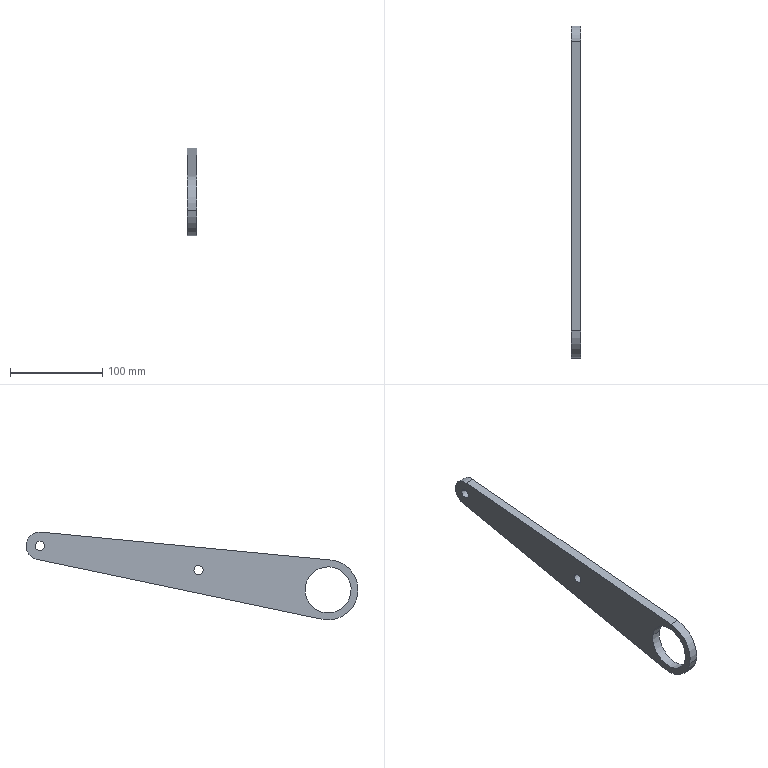Part | NX | features _-17372000 2 | 1 solid | 13 faces | box 10 x 359.893 x 95.107 mm | volume 149250 mm3 | cylinder 9 | plane 4 | commonest cylinder face diameters 10 x4 50 x2 65 x2 30 x1
STEP:
#1=CARTESIAN_POINT('',(-12.5,-285.515,-699.296));
#2=VERTEX_POINT('',#1);
#3=CARTESIAN_POINT('',(-12.5,-236.085,-691.763));
#4=VERTEX_POINT('',#3);
#5=CARTESIAN_POINT('',(-12.5,-260.8,-695.529));
#6=DIRECTION('',(1.,0.,0.));
#7=DIRECTION('',(0.,-0.9886,-0.1507));
#8=AXIS2_PLACEMENT_3D('',#5,#6,#7);
#9=CIRCLE('',#8,25.);
#10=EDGE_CURVE('',#2,#4,#9,.T.);
#11=ORIENTED_EDGE('',*,*,#10,.F.);
#12=CARTESIAN_POINT('',(-2.5,-285.515,-699.296));
#13=VERTEX_POINT('',#12);
#14=CARTESIAN_POINT('',(-2.5,-285.515,-699.296));
#15=DIRECTION('',(-1.,0.,0.));
#16=VECTOR('',#15,1000.);
#17=LINE('',#14,#16);
#18=EDGE_CURVE('',#2,#13,#17,.F.);
#19=ORIENTED_EDGE('',*,*,#18,.T.);
#20=CARTESIAN_POINT('',(-2.5,-236.085,-691.763));
#21=VERTEX_POINT('',#20);
#22=CARTESIAN_POINT('',(-2.5,-260.8,-695.529));
#23=DIRECTION('',(-1.,0.,0.));
#24=DIRECTION('',(0.,0.9886,0.1507));
#25=AXIS2_PLACEMENT_3D('',#22,#23,#24);
#26=CIRCLE('',#25,25.);
#27=EDGE_CURVE('',#21,#13,#26,.T.);
#28=ORIENTED_EDGE('',*,*,#27,.F.);
#29=CARTESIAN_POINT('',(-2.5,-236.085,-691.763));
#30=DIRECTION('',(-1.,0.,0.));
#31=VECTOR('',#30,1000.);
#32=LINE('',#29,#31);
#33=EDGE_CURVE('',#21,#4,#32,.T.);
#34=ORIENTED_EDGE('',*,*,#33,.T.);
#35=EDGE_LOOP('',(#11,#19,#28,#34));
#36=FACE_BOUND('',#35,.T.);
#37=CARTESIAN_POINT('',(-12.5,-260.8,-695.529));
#38=DIRECTION('',(1.,0.,0.));
#39=DIRECTION('',(0.,-0.9886,-0.1507));
#40=AXIS2_PLACEMENT_3D('',#37,#38,#39);
#41=CYLINDRICAL_SURFACE('',#40,25.);
#42=ADVANCED_FACE('',(#36),#41,.F.);
#43=ORIENTED_EDGE('',*,*,#33,.F.);
#44=CARTESIAN_POINT('',(-2.5,-260.8,-695.529));
#45=DIRECTION('',(-1.,0.,0.));
#46=DIRECTION('',(0.,-0.9886,-0.1507));
#47=AXIS2_PLACEMENT_3D('',#44,#45,#46);
#48=CIRCLE('',#47,25.);
#49=EDGE_CURVE('',#13,#21,#48,.T.);
#50=ORIENTED_EDGE('',*,*,#49,.F.);
#51=ORIENTED_EDGE('',*,*,#18,.F.);
#52=CARTESIAN_POINT('',(-12.5,-260.8,-695.529));
#53=DIRECTION('',(1.,0.,0.));
#54=DIRECTION('',(0.,0.9886,0.1507));
#55=AXIS2_PLACEMENT_3D('',#52,#53,#54);
#56=CIRCLE('',#55,25.);
#57=EDGE_CURVE('',#4,#2,#56,.T.);
#58=ORIENTED_EDGE('',*,*,#57,.F.);
#59=EDGE_LOOP('',(#43,#50,#51,#58));
#60=FACE_BOUND('',#59,.T.);
#61=CARTESIAN_POINT('',(-12.5,-260.8,-695.529));
#62=DIRECTION('',(1.,0.,0.));
#63=DIRECTION('',(0.,-0.9886,-0.1507));
#64=AXIS2_PLACEMENT_3D('',#61,#62,#63);
#65=CYLINDRICAL_SURFACE('',#64,25.);
#66=ADVANCED_FACE('',(#60),#65,.F.);
#67=CARTESIAN_POINT('',(-12.5,-125.364,-674.89));
#68=VERTEX_POINT('',#67);
#69=CARTESIAN_POINT('',(-12.5,-115.478,-673.383));
#70=VERTEX_POINT('',#69);
#71=CARTESIAN_POINT('',(-12.5,-120.421,-674.136));
#72=DIRECTION('',(1.,0.,0.));
#73=DIRECTION('',(0.,-0.9886,-0.1507));
#74=AXIS2_PLACEMENT_3D('',#71,#72,#73);
#75=CIRCLE('',#74,5.);
#76=EDGE_CURVE('',#68,#70,#75,.T.);
#77=ORIENTED_EDGE('',*,*,#76,.F.);
#78=CARTESIAN_POINT('',(-2.5,-125.364,-674.89));
#79=VERTEX_POINT('',#78);
#80=CARTESIAN_POINT('',(-2.5,-125.364,-674.89));
#81=DIRECTION('',(-1.,0.,0.));
#82=VECTOR('',#81,1000.);
#83=LINE('',#80,#82);
#84=EDGE_CURVE('',#68,#79,#83,.F.);
#85=ORIENTED_EDGE('',*,*,#84,.T.);
#86=CARTESIAN_POINT('',(-2.5,-115.478,-673.383));
#87=VERTEX_POINT('',#86);
#88=CARTESIAN_POINT('',(-2.5,-120.421,-674.136));
#89=DIRECTION('',(-1.,0.,0.));
#90=DIRECTION('',(0.,0.9886,0.1507));
#91=AXIS2_PLACEMENT_3D('',#88,#89,#90);
#92=CIRCLE('',#91,5.);
#93=EDGE_CURVE('',#87,#79,#92,.T.);
#94=ORIENTED_EDGE('',*,*,#93,.F.);
#95=CARTESIAN_POINT('',(-2.5,-115.478,-673.383));
#96=DIRECTION('',(-1.,0.,0.));
#97=VECTOR('',#96,1000.);
#98=LINE('',#95,#97);
#99=EDGE_CURVE('',#87,#70,#98,.T.);
#100=ORIENTED_EDGE('',*,*,#99,.T.);
#101=EDGE_LOOP('',(#77,#85,#94,#100));
#102=FACE_BOUND('',#101,.T.);
#103=CARTESIAN_POINT('',(-12.5,-120.421,-674.136));
#104=DIRECTION('',(1.,0.,0.));
#105=DIRECTION('',(0.,-0.9886,-0.1507));
#106=AXIS2_PLACEMENT_3D('',#103,#104,#105);
#107=CYLINDRICAL_SURFACE('',#106,5.);
#108=ADVANCED_FACE('',(#102),#107,.F.);
#109=ORIENTED_EDGE('',*,*,#99,.F.);
#110=CARTESIAN_POINT('',(-2.5,-120.421,-674.136));
#111=DIRECTION('',(-1.,0.,0.));
#112=DIRECTION('',(0.,-0.9886,-0.1507));
#113=AXIS2_PLACEMENT_3D('',#110,#111,#112);
#114=CIRCLE('',#113,5.);
#115=EDGE_CURVE('',#79,#87,#114,.T.);
#116=ORIENTED_EDGE('',*,*,#115,.F.);
#117=ORIENTED_EDGE('',*,*,#84,.F.);
#118=CARTESIAN_POINT('',(-12.5,-120.421,-674.136));
#119=DIRECTION('',(1.,0.,0.));
#120=DIRECTION('',(0.,0.9886,0.1507));
#121=AXIS2_PLACEMENT_3D('',#118,#119,#120);
#122=CIRCLE('',#121,5.);
#123=EDGE_CURVE('',#70,#68,#122,.T.);
#124=ORIENTED_EDGE('',*,*,#123,.F.);
#125=EDGE_LOOP('',(#109,#116,#117,#124));
#126=FACE_BOUND('',#125,.T.);
#127=CARTESIAN_POINT('',(-12.5,-120.421,-674.136));
#128=DIRECTION('',(1.,0.,0.));
#129=DIRECTION('',(0.,-0.9886,-0.1507));
#130=AXIS2_PLACEMENT_3D('',#127,#128,#129);
#131=CYLINDRICAL_SURFACE('',#130,5.);
#132=ADVANCED_FACE('',(#126),#131,.F.);
#133=CARTESIAN_POINT('',(-12.5,46.65,-648.676));
#134=VERTEX_POINT('',#133);
#135=CARTESIAN_POINT('',(-12.5,56.536,-647.169));
#136=VERTEX_POINT('',#135);
#137=CARTESIAN_POINT('',(-12.5,51.593,-647.922));
#138=DIRECTION('',(1.,0.,0.));
#139=DIRECTION('',(0.,-0.9886,-0.1507));
#140=AXIS2_PLACEMENT_3D('',#137,#138,#139);
#141=CIRCLE('',#140,5.);
#142=EDGE_CURVE('',#134,#136,#141,.T.);
#143=ORIENTED_EDGE('',*,*,#142,.F.);
#144=CARTESIAN_POINT('',(-2.5,46.65,-648.676));
#145=VERTEX_POINT('',#144);
#146=CARTESIAN_POINT('',(-2.5,46.65,-648.676));
#147=DIRECTION('',(-1.,0.,0.));
#148=VECTOR('',#147,1000.);
#149=LINE('',#146,#148);
#150=EDGE_CURVE('',#145,#134,#149,.T.);
#151=ORIENTED_EDGE('',*,*,#150,.F.);
#152=CARTESIAN_POINT('',(-2.5,56.536,-647.169));
#153=VERTEX_POINT('',#152);
#154=CARTESIAN_POINT('',(-2.5,51.593,-647.922));
#155=DIRECTION('',(-1.,0.,0.));
#156=DIRECTION('',(0.,0.9886,0.1507));
#157=AXIS2_PLACEMENT_3D('',#154,#155,#156);
#158=CIRCLE('',#157,5.);
#159=EDGE_CURVE('',#153,#145,#158,.T.);
#160=ORIENTED_EDGE('',*,*,#159,.F.);
#161=CARTESIAN_POINT('',(-2.5,56.536,-647.169));
#162=DIRECTION('',(-1.,0.,0.));
#163=VECTOR('',#162,1000.);
#164=LINE('',#161,#163);
#165=EDGE_CURVE('',#136,#153,#164,.F.);
#166=ORIENTED_EDGE('',*,*,#165,.F.);
#167=EDGE_LOOP('',(#143,#151,#160,#166));
#168=FACE_BOUND('',#167,.T.);
#169=CARTESIAN_POINT('',(-12.5,51.593,-647.922));
#170=DIRECTION('',(1.,0.,0.));
#171=DIRECTION('',(0.,-0.9886,-0.1507));
#172=AXIS2_PLACEMENT_3D('',#169,#170,#171);
#173=CYLINDRICAL_SURFACE('',#172,5.);
#174=ADVANCED_FACE('',(#168),#173,.F.);
#175=ORIENTED_EDGE('',*,*,#165,.T.);
#176=CARTESIAN_POINT('',(-2.5,51.593,-647.922));
#177=DIRECTION('',(-1.,0.,0.));
#178=DIRECTION('',(0.,-0.9886,-0.1507));
#179=AXIS2_PLACEMENT_3D('',#176,#177,#178);
#180=CIRCLE('',#179,5.);
#181=EDGE_CURVE('',#145,#153,#180,.T.);
#182=ORIENTED_EDGE('',*,*,#181,.F.);
#183=ORIENTED_EDGE('',*,*,#150,.T.);
#184=CARTESIAN_POINT('',(-12.5,51.593,-647.922));
#185=DIRECTION('',(1.,0.,0.));
#186=DIRECTION('',(0.,0.9886,0.1507));
#187=AXIS2_PLACEMENT_3D('',#184,#185,#186);
#188=CIRCLE('',#187,5.);
#189=EDGE_CURVE('',#136,#134,#188,.T.);
#190=ORIENTED_EDGE('',*,*,#189,.F.);
#191=EDGE_LOOP('',(#175,#182,#183,#190));
#192=FACE_BOUND('',#191,.T.);
#193=CARTESIAN_POINT('',(-12.5,51.593,-647.922));
#194=DIRECTION('',(1.,0.,0.));
#195=DIRECTION('',(0.,-0.9886,-0.1507));
#196=AXIS2_PLACEMENT_3D('',#193,#194,#195);
#197=CYLINDRICAL_SURFACE('',#196,5.);
#198=ADVANCED_FACE('',(#192),#197,.F.);
#199=CARTESIAN_POINT('',(-12.5,-254.132,-727.338));
#200=VERTEX_POINT('',#199);
#201=CARTESIAN_POINT('',(-2.5,-254.132,-727.338));
#202=VERTEX_POINT('',#201);
#203=CARTESIAN_POINT('',(-12.5,-254.132,-727.338));
#204=DIRECTION('',(1.,0.,0.));
#205=VECTOR('',#204,1000.);
#206=LINE('',#203,#205);
#207=EDGE_CURVE('',#200,#202,#206,.T.);
#208=ORIENTED_EDGE('',*,*,#207,.F.);
#209=CARTESIAN_POINT('',(-12.5,54.671,-662.603));
#210=VERTEX_POINT('',#209);
#211=CARTESIAN_POINT('',(-12.5,54.671,-662.603));
#212=DIRECTION('',(0.,-0.9787,-0.2052));
#213=VECTOR('',#212,1000.);
#214=LINE('',#211,#213);
#215=EDGE_CURVE('',#210,#200,#214,.T.);
#216=ORIENTED_EDGE('',*,*,#215,.F.);
#217=CARTESIAN_POINT('',(-2.5,54.671,-662.603));
#218=VERTEX_POINT('',#217);
#219=CARTESIAN_POINT('',(-2.5,54.671,-662.603));
#220=DIRECTION('',(-1.,0.,0.));
#221=VECTOR('',#220,1000.);
#222=LINE('',#219,#221);
#223=EDGE_CURVE('',#218,#210,#222,.T.);
#224=ORIENTED_EDGE('',*,*,#223,.F.);
#225=CARTESIAN_POINT('',(-2.5,-254.132,-727.338));
#226=DIRECTION('',(0.,0.9787,0.2052));
#227=VECTOR('',#226,1000.);
#228=LINE('',#225,#227);
#229=EDGE_CURVE('',#202,#218,#228,.T.);
#230=ORIENTED_EDGE('',*,*,#229,.F.);
#231=EDGE_LOOP('',(#208,#216,#224,#230));
#232=FACE_BOUND('',#231,.T.);
#233=CARTESIAN_POINT('',(-12.5,54.671,-662.603));
#234=DIRECTION('',(0.,-0.2052,0.9787));
#235=DIRECTION('',(0.,0.9787,0.2052));
#236=AXIS2_PLACEMENT_3D('',#233,#234,#235);
#237=PLANE('',#236);
#238=ADVANCED_FACE('',(#232),#237,.F.);
#239=ORIENTED_EDGE('',*,*,#223,.T.);
#240=CARTESIAN_POINT('',(-12.5,50.158,-632.991));
#241=VERTEX_POINT('',#240);
#242=CARTESIAN_POINT('',(-12.5,51.593,-647.922));
#243=DIRECTION('',(-1.,0.,0.));
#244=DIRECTION('',(0.,-0.09568,0.9954));
#245=AXIS2_PLACEMENT_3D('',#242,#243,#244);
#246=CIRCLE('',#245,15.);
#247=EDGE_CURVE('',#241,#210,#246,.T.);
#248=ORIENTED_EDGE('',*,*,#247,.F.);
#249=CARTESIAN_POINT('',(-2.5,50.158,-632.991));
#250=VERTEX_POINT('',#249);
#251=CARTESIAN_POINT('',(-12.5,50.158,-632.991));
#252=DIRECTION('',(1.,0.,0.));
#253=VECTOR('',#252,1000.);
#254=LINE('',#251,#253);
#255=EDGE_CURVE('',#241,#250,#254,.T.);
#256=ORIENTED_EDGE('',*,*,#255,.T.);
#257=CARTESIAN_POINT('',(-2.5,51.593,-647.922));
#258=DIRECTION('',(1.,0.,0.));
#259=DIRECTION('',(0.,0.2052,-0.9787));
#260=AXIS2_PLACEMENT_3D('',#257,#258,#259);
#261=CIRCLE('',#260,15.);
#262=EDGE_CURVE('',#218,#250,#261,.T.);
#263=ORIENTED_EDGE('',*,*,#262,.F.);
#264=EDGE_LOOP('',(#239,#248,#256,#263));
#265=FACE_BOUND('',#264,.T.);
#266=CARTESIAN_POINT('',(-12.5,51.593,-647.922));
#267=DIRECTION('',(1.,0.,0.));
#268=DIRECTION('',(0.,-0.9886,-0.1507));
#269=AXIS2_PLACEMENT_3D('',#266,#267,#268);
#270=CYLINDRICAL_SURFACE('',#269,15.);
#271=ADVANCED_FACE('',(#265),#270,.T.);
#272=ORIENTED_EDGE('',*,*,#27,.T.);
#273=ORIENTED_EDGE('',*,*,#49,.T.);
#274=EDGE_LOOP('',(#272,#273));
#275=FACE_BOUND('',#274,.T.);
#276=ORIENTED_EDGE('',*,*,#93,.T.);
#277=ORIENTED_EDGE('',*,*,#115,.T.);
#278=EDGE_LOOP('',(#276,#277));
#279=FACE_BOUND('',#278,.T.);
#280=ORIENTED_EDGE('',*,*,#159,.T.);
#281=ORIENTED_EDGE('',*,*,#181,.T.);
#282=EDGE_LOOP('',(#280,#281));
#283=FACE_BOUND('',#282,.T.);
#284=ORIENTED_EDGE('',*,*,#229,.T.);
#285=ORIENTED_EDGE('',*,*,#262,.T.);
#286=CARTESIAN_POINT('',(-2.5,-263.909,-663.179));
#287=VERTEX_POINT('',#286);
#288=CARTESIAN_POINT('',(-2.5,50.158,-632.991));
#289=DIRECTION('',(0.,-0.9954,-0.09568));
#290=VECTOR('',#289,1000.);
#291=LINE('',#288,#290);
#292=EDGE_CURVE('',#250,#287,#291,.T.);
#293=ORIENTED_EDGE('',*,*,#292,.T.);
#294=CARTESIAN_POINT('',(-2.5,-292.929,-700.426));
#295=VERTEX_POINT('',#294);
#296=CARTESIAN_POINT('',(-2.5,-260.8,-695.529));
#297=DIRECTION('',(1.,0.,0.));
#298=DIRECTION('',(0.,-0.09568,0.9954));
#299=AXIS2_PLACEMENT_3D('',#296,#297,#298);
#300=CIRCLE('',#299,32.5);
#301=EDGE_CURVE('',#287,#295,#300,.T.);
#302=ORIENTED_EDGE('',*,*,#301,.T.);
#303=CARTESIAN_POINT('',(-2.5,-260.8,-695.529));
#304=DIRECTION('',(1.,0.,0.));
#305=DIRECTION('',(0.,-0.9886,-0.1507));
#306=AXIS2_PLACEMENT_3D('',#303,#304,#305);
#307=CIRCLE('',#306,32.5);
#308=EDGE_CURVE('',#295,#202,#307,.T.);
#309=ORIENTED_EDGE('',*,*,#308,.T.);
#310=EDGE_LOOP('',(#284,#285,#293,#302,#309));
#311=FACE_BOUND('',#310,.T.);
#312=CARTESIAN_POINT('',(-2.5,-260.8,-695.529));
#313=DIRECTION('',(-1.,0.,0.));
#314=DIRECTION('',(0.,0.9886,0.1507));
#315=AXIS2_PLACEMENT_3D('',#312,#313,#314);
#316=PLANE('',#315);
#317=ADVANCED_FACE('',(#275,#279,#283,#311),#316,.F.);
#318=ORIENTED_EDGE('',*,*,#255,.F.);
#319=CARTESIAN_POINT('',(-12.5,-263.909,-663.179));
#320=VERTEX_POINT('',#319);
#321=CARTESIAN_POINT('',(-12.5,-263.909,-663.179));
#322=DIRECTION('',(0.,0.9954,0.09568));
#323=VECTOR('',#322,1000.);
#324=LINE('',#321,#323);
#325=EDGE_CURVE('',#320,#241,#324,.T.);
#326=ORIENTED_EDGE('',*,*,#325,.F.);
#327=CARTESIAN_POINT('',(-2.5,-263.909,-663.179));
#328=DIRECTION('',(-1.,0.,0.));
#329=VECTOR('',#328,1000.);
#330=LINE('',#327,#329);
#331=EDGE_CURVE('',#287,#320,#330,.T.);
#332=ORIENTED_EDGE('',*,*,#331,.F.);
#333=ORIENTED_EDGE('',*,*,#292,.F.);
#334=EDGE_LOOP('',(#318,#326,#332,#333));
#335=FACE_BOUND('',#334,.T.);
#336=CARTESIAN_POINT('',(-12.5,-263.909,-663.179));
#337=DIRECTION('',(0.,0.09568,-0.9954));
#338=DIRECTION('',(0.,-0.9954,-0.09568));
#339=AXIS2_PLACEMENT_3D('',#336,#337,#338);
#340=PLANE('',#339);
#341=ADVANCED_FACE('',(#335),#340,.F.);
#342=CARTESIAN_POINT('',(-12.5,-292.929,-700.426));
#343=VERTEX_POINT('',#342);
#344=CARTESIAN_POINT('',(-2.5,-292.929,-700.426));
#345=DIRECTION('',(-1.,0.,0.));
#346=VECTOR('',#345,1000.);
#347=LINE('',#344,#346);
#348=EDGE_CURVE('',#295,#343,#347,.T.);
#349=ORIENTED_EDGE('',*,*,#348,.F.);
#350=ORIENTED_EDGE('',*,*,#301,.F.);
#351=ORIENTED_EDGE('',*,*,#331,.T.);
#352=CARTESIAN_POINT('',(-12.5,-260.8,-695.529));
#353=DIRECTION('',(-1.,0.,0.));
#354=DIRECTION('',(0.,-0.9886,-0.1507));
#355=AXIS2_PLACEMENT_3D('',#352,#353,#354);
#356=CIRCLE('',#355,32.5);
#357=EDGE_CURVE('',#343,#320,#356,.T.);
#358=ORIENTED_EDGE('',*,*,#357,.F.);
#359=EDGE_LOOP('',(#349,#350,#351,#358));
#360=FACE_BOUND('',#359,.T.);
#361=CARTESIAN_POINT('',(-12.5,-260.8,-695.529));
#362=DIRECTION('',(1.,0.,0.));
#363=DIRECTION('',(0.,-0.9886,-0.1507));
#364=AXIS2_PLACEMENT_3D('',#361,#362,#363);
#365=CYLINDRICAL_SURFACE('',#364,32.5);
#366=ADVANCED_FACE('',(#360),#365,.T.);
#367=CARTESIAN_POINT('',(-12.5,-260.8,-695.529));
#368=DIRECTION('',(-1.,0.,0.));
#369=DIRECTION('',(0.,0.2052,-0.9787));
#370=AXIS2_PLACEMENT_3D('',#367,#368,#369);
#371=CIRCLE('',#370,32.5);
#372=EDGE_CURVE('',#200,#343,#371,.T.);
#373=ORIENTED_EDGE('',*,*,#372,.F.);
#374=ORIENTED_EDGE('',*,*,#207,.T.);
#375=ORIENTED_EDGE('',*,*,#308,.F.);
#376=ORIENTED_EDGE('',*,*,#348,.T.);
#377=EDGE_LOOP('',(#373,#374,#375,#376));
#378=FACE_BOUND('',#377,.T.);
#379=CARTESIAN_POINT('',(-12.5,-260.8,-695.529));
#380=DIRECTION('',(1.,0.,0.));
#381=DIRECTION('',(0.,-0.9886,-0.1507));
#382=AXIS2_PLACEMENT_3D('',#379,#380,#381);
#383=CYLINDRICAL_SURFACE('',#382,32.5);
#384=ADVANCED_FACE('',(#378),#383,.T.);
#385=ORIENTED_EDGE('',*,*,#10,.T.);
#386=ORIENTED_EDGE('',*,*,#57,.T.);
#387=EDGE_LOOP('',(#385,#386));
#388=FACE_BOUND('',#387,.T.);
#389=ORIENTED_EDGE('',*,*,#76,.T.);
#390=ORIENTED_EDGE('',*,*,#123,.T.);
#391=EDGE_LOOP('',(#389,#390));
#392=FACE_BOUND('',#391,.T.);
#393=ORIENTED_EDGE('',*,*,#142,.T.);
#394=ORIENTED_EDGE('',*,*,#189,.T.);
#395=EDGE_LOOP('',(#393,#394));
#396=FACE_BOUND('',#395,.T.);
#397=ORIENTED_EDGE('',*,*,#357,.T.);
#398=ORIENTED_EDGE('',*,*,#325,.T.);
#399=ORIENTED_EDGE('',*,*,#247,.T.);
#400=ORIENTED_EDGE('',*,*,#215,.T.);
#401=ORIENTED_EDGE('',*,*,#372,.T.);
#402=EDGE_LOOP('',(#397,#398,#399,#400,#401));
#403=FACE_BOUND('',#402,.T.);
#404=CARTESIAN_POINT('',(-12.5,-260.8,-695.529));
#405=DIRECTION('',(-1.,0.,0.));
#406=DIRECTION('',(0.,0.9886,0.1507));
#407=AXIS2_PLACEMENT_3D('',#404,#405,#406);
#408=PLANE('',#407);
#409=ADVANCED_FACE('',(#388,#392,#396,#403),#408,.T.);
#410=CLOSED_SHELL('',(#42,#66,#108,#132,#174,#198,#238,#271,#317,#341,#366,#384,#409));
#411=MANIFOLD_SOLID_BREP('',#410);
#412=(LENGTH_UNIT()NAMED_UNIT(*)SI_UNIT(.MILLI.,.METRE.));
#413=UNCERTAINTY_MEASURE_WITH_UNIT(LENGTH_MEASURE(0.00001),#412,'','');
#414=(NAMED_UNIT(*)PLANE_ANGLE_UNIT()SI_UNIT($,.RADIAN.));
#415=(NAMED_UNIT(*)SI_UNIT($,.STERADIAN.)SOLID_ANGLE_UNIT());
#416=(GEOMETRIC_REPRESENTATION_CONTEXT(3)GLOBAL_UNCERTAINTY_ASSIGNED_CONTEXT((#413))GLOBAL_UNIT_ASSIGNED_CONTEXT((#412,#414,#415))REPRESENTATION_CONTEXT('',''));
#417=ADVANCED_BREP_SHAPE_REPRESENTATION('',(#411),#416);